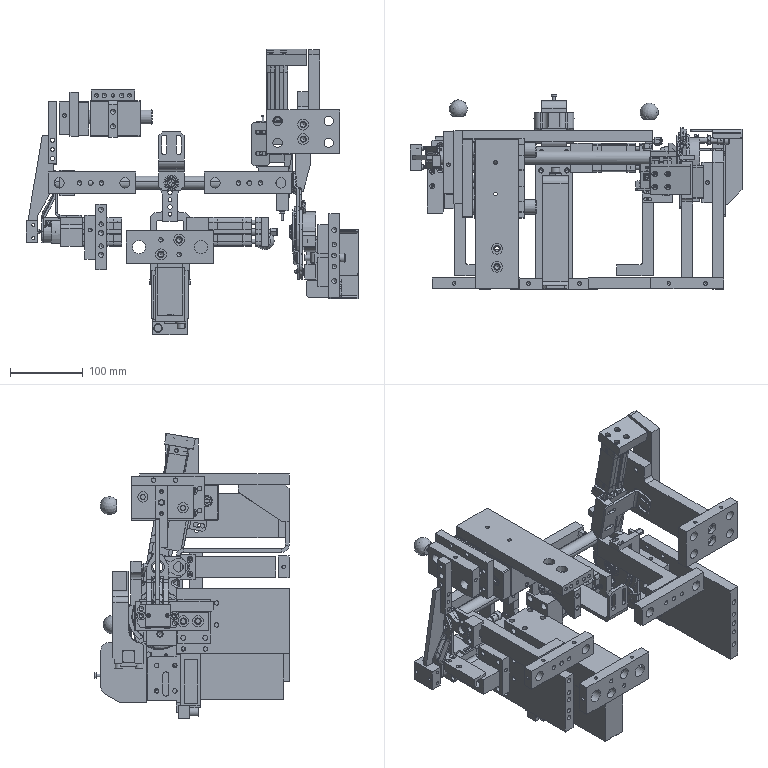Part | NX | features BREP 91 | 182 solids | 13276 faces | volume 4410668 mm3 | cylinder 4903 | plane 4568 | spline 1744 | cone 1034 | torus 889 | sphere 138 | commonest cylinder face diameters 0.3 x676 0.6 x576 1 x256 6 x177 4 x173 2 x160